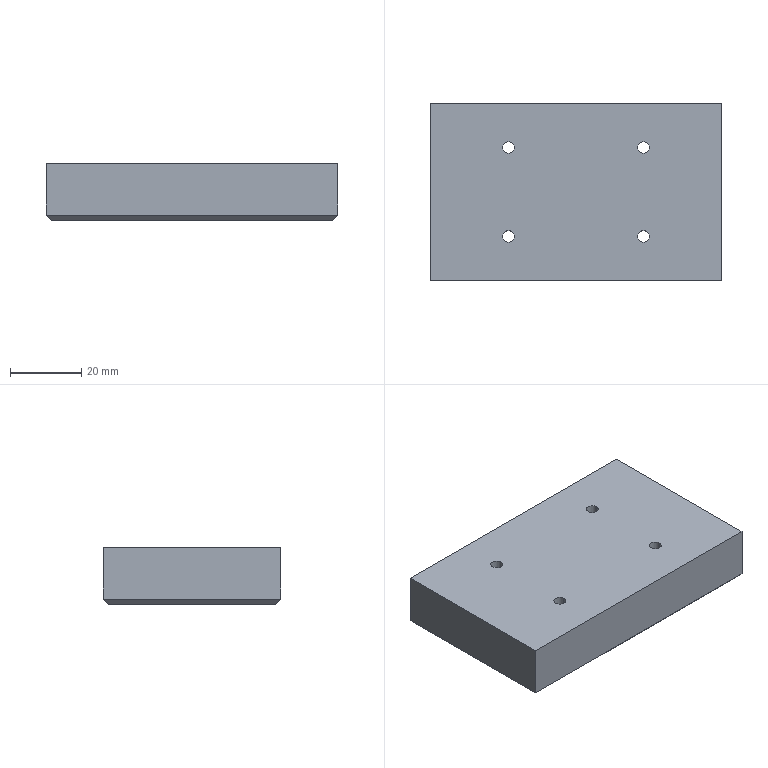Part | SolidWorks | features 3DProfileFeature 1, Chamfer 1, Extrusion 1, HoleWzd 1, LPattern 1 | 1 solid | 18 faces | box 82 x 50 x 16 mm | volume 64760 mm3 | plane 10 | cylinder 8 | commonest cylinder face diameters 3.3 x8
STEP:
#1=CARTESIAN_POINT('',(-17.35,-12.5,16.));
#2=VERTEX_POINT('',#1);
#3=CARTESIAN_POINT('',(-20.65,-12.5,16.));
#4=VERTEX_POINT('',#3);
#5=CARTESIAN_POINT('',(-19.,-12.5,16.));
#6=DIRECTION('',(0.,0.,-1.));
#7=DIRECTION('',(-1.,0.,0.));
#8=AXIS2_PLACEMENT_3D('',#5,#6,#7);
#9=CIRCLE('',#8,1.65);
#10=EDGE_CURVE('',#2,#4,#9,.T.);
#11=ORIENTED_EDGE('',*,*,#10,.F.);
#12=CARTESIAN_POINT('',(-17.35,-12.5,0.));
#13=VERTEX_POINT('',#12);
#14=CARTESIAN_POINT('',(-17.35,-12.5,0.));
#15=DIRECTION('',(0.,0.,-1.));
#16=VECTOR('',#15,1000.);
#17=LINE('',#14,#16);
#18=EDGE_CURVE('',#2,#13,#17,.T.);
#19=ORIENTED_EDGE('',*,*,#18,.T.);
#20=CARTESIAN_POINT('',(-20.65,-12.5,0.));
#21=VERTEX_POINT('',#20);
#22=CARTESIAN_POINT('',(-19.,-12.5,0.));
#23=DIRECTION('',(0.,0.,-1.));
#24=DIRECTION('',(-1.,0.,0.));
#25=AXIS2_PLACEMENT_3D('',#22,#23,#24);
#26=CIRCLE('',#25,1.65);
#27=EDGE_CURVE('',#13,#21,#26,.T.);
#28=ORIENTED_EDGE('',*,*,#27,.T.);
#29=CARTESIAN_POINT('',(-20.65,-12.5,0.));
#30=DIRECTION('',(0.,0.,-1.));
#31=VECTOR('',#30,1000.);
#32=LINE('',#29,#31);
#33=EDGE_CURVE('',#4,#21,#32,.T.);
#34=ORIENTED_EDGE('',*,*,#33,.F.);
#35=EDGE_LOOP('',(#11,#19,#28,#34));
#36=FACE_OUTER_BOUND('',#35,.T.);
#37=CARTESIAN_POINT('',(-19.,-12.5,0.));
#38=DIRECTION('',(0.,0.,-1.));
#39=DIRECTION('',(-1.,0.,0.));
#40=AXIS2_PLACEMENT_3D('',#37,#38,#39);
#41=CYLINDRICAL_SURFACE('',#40,1.65);
#42=ADVANCED_FACE('',(#36),#41,.F.);
#43=CARTESIAN_POINT('',(-17.35,12.5,16.));
#44=VERTEX_POINT('',#43);
#45=CARTESIAN_POINT('',(-20.65,12.5,16.));
#46=VERTEX_POINT('',#45);
#47=CARTESIAN_POINT('',(-19.,12.5,16.));
#48=DIRECTION('',(0.,0.,-1.));
#49=DIRECTION('',(-1.,0.,0.));
#50=AXIS2_PLACEMENT_3D('',#47,#48,#49);
#51=CIRCLE('',#50,1.65);
#52=EDGE_CURVE('',#44,#46,#51,.T.);
#53=ORIENTED_EDGE('',*,*,#52,.F.);
#54=CARTESIAN_POINT('',(-17.35,12.5,0.));
#55=VERTEX_POINT('',#54);
#56=CARTESIAN_POINT('',(-17.35,12.5,0.));
#57=DIRECTION('',(0.,0.,-1.));
#58=VECTOR('',#57,1000.);
#59=LINE('',#56,#58);
#60=EDGE_CURVE('',#44,#55,#59,.T.);
#61=ORIENTED_EDGE('',*,*,#60,.T.);
#62=CARTESIAN_POINT('',(-20.65,12.5,0.));
#63=VERTEX_POINT('',#62);
#64=CARTESIAN_POINT('',(-19.,12.5,0.));
#65=DIRECTION('',(0.,0.,-1.));
#66=DIRECTION('',(-1.,0.,0.));
#67=AXIS2_PLACEMENT_3D('',#64,#65,#66);
#68=CIRCLE('',#67,1.65);
#69=EDGE_CURVE('',#55,#63,#68,.T.);
#70=ORIENTED_EDGE('',*,*,#69,.T.);
#71=CARTESIAN_POINT('',(-20.65,12.5,0.));
#72=DIRECTION('',(0.,0.,-1.));
#73=VECTOR('',#72,1000.);
#74=LINE('',#71,#73);
#75=EDGE_CURVE('',#46,#63,#74,.T.);
#76=ORIENTED_EDGE('',*,*,#75,.F.);
#77=EDGE_LOOP('',(#53,#61,#70,#76));
#78=FACE_OUTER_BOUND('',#77,.T.);
#79=CARTESIAN_POINT('',(-19.,12.5,0.));
#80=DIRECTION('',(0.,0.,-1.));
#81=DIRECTION('',(-1.,0.,0.));
#82=AXIS2_PLACEMENT_3D('',#79,#80,#81);
#83=CYLINDRICAL_SURFACE('',#82,1.65);
#84=ADVANCED_FACE('',(#78),#83,.F.);
#85=CARTESIAN_POINT('',(20.65,-12.5,16.));
#86=VERTEX_POINT('',#85);
#87=CARTESIAN_POINT('',(17.35,-12.5,16.));
#88=VERTEX_POINT('',#87);
#89=CARTESIAN_POINT('',(19.,-12.5,16.));
#90=DIRECTION('',(0.,0.,-1.));
#91=DIRECTION('',(-1.,0.,0.));
#92=AXIS2_PLACEMENT_3D('',#89,#90,#91);
#93=CIRCLE('',#92,1.65);
#94=EDGE_CURVE('',#86,#88,#93,.T.);
#95=ORIENTED_EDGE('',*,*,#94,.F.);
#96=CARTESIAN_POINT('',(20.65,-12.5,0.));
#97=VERTEX_POINT('',#96);
#98=CARTESIAN_POINT('',(20.65,-12.5,0.));
#99=DIRECTION('',(0.,0.,-1.));
#100=VECTOR('',#99,1000.);
#101=LINE('',#98,#100);
#102=EDGE_CURVE('',#86,#97,#101,.T.);
#103=ORIENTED_EDGE('',*,*,#102,.T.);
#104=CARTESIAN_POINT('',(17.35,-12.5,0.));
#105=VERTEX_POINT('',#104);
#106=CARTESIAN_POINT('',(19.,-12.5,0.));
#107=DIRECTION('',(0.,0.,-1.));
#108=DIRECTION('',(-1.,0.,0.));
#109=AXIS2_PLACEMENT_3D('',#106,#107,#108);
#110=CIRCLE('',#109,1.65);
#111=EDGE_CURVE('',#97,#105,#110,.T.);
#112=ORIENTED_EDGE('',*,*,#111,.T.);
#113=CARTESIAN_POINT('',(17.35,-12.5,0.));
#114=DIRECTION('',(0.,0.,-1.));
#115=VECTOR('',#114,1000.);
#116=LINE('',#113,#115);
#117=EDGE_CURVE('',#88,#105,#116,.T.);
#118=ORIENTED_EDGE('',*,*,#117,.F.);
#119=EDGE_LOOP('',(#95,#103,#112,#118));
#120=FACE_OUTER_BOUND('',#119,.T.);
#121=CARTESIAN_POINT('',(19.,-12.5,0.));
#122=DIRECTION('',(0.,0.,-1.));
#123=DIRECTION('',(-1.,0.,0.));
#124=AXIS2_PLACEMENT_3D('',#121,#122,#123);
#125=CYLINDRICAL_SURFACE('',#124,1.65);
#126=ADVANCED_FACE('',(#120),#125,.F.);
#127=CARTESIAN_POINT('',(20.65,12.5,16.));
#128=VERTEX_POINT('',#127);
#129=CARTESIAN_POINT('',(17.35,12.5,16.));
#130=VERTEX_POINT('',#129);
#131=CARTESIAN_POINT('',(19.,12.5,16.));
#132=DIRECTION('',(0.,0.,-1.));
#133=DIRECTION('',(-1.,0.,0.));
#134=AXIS2_PLACEMENT_3D('',#131,#132,#133);
#135=CIRCLE('',#134,1.65);
#136=EDGE_CURVE('',#128,#130,#135,.T.);
#137=ORIENTED_EDGE('',*,*,#136,.F.);
#138=CARTESIAN_POINT('',(20.65,12.5,0.));
#139=VERTEX_POINT('',#138);
#140=CARTESIAN_POINT('',(20.65,12.5,0.));
#141=DIRECTION('',(0.,0.,-1.));
#142=VECTOR('',#141,1000.);
#143=LINE('',#140,#142);
#144=EDGE_CURVE('',#128,#139,#143,.T.);
#145=ORIENTED_EDGE('',*,*,#144,.T.);
#146=CARTESIAN_POINT('',(17.35,12.5,0.));
#147=VERTEX_POINT('',#146);
#148=CARTESIAN_POINT('',(19.,12.5,0.));
#149=DIRECTION('',(0.,0.,-1.));
#150=DIRECTION('',(-1.,0.,0.));
#151=AXIS2_PLACEMENT_3D('',#148,#149,#150);
#152=CIRCLE('',#151,1.65);
#153=EDGE_CURVE('',#139,#147,#152,.T.);
#154=ORIENTED_EDGE('',*,*,#153,.T.);
#155=CARTESIAN_POINT('',(17.35,12.5,0.));
#156=DIRECTION('',(0.,0.,-1.));
#157=VECTOR('',#156,1000.);
#158=LINE('',#155,#157);
#159=EDGE_CURVE('',#130,#147,#158,.T.);
#160=ORIENTED_EDGE('',*,*,#159,.F.);
#161=EDGE_LOOP('',(#137,#145,#154,#160));
#162=FACE_OUTER_BOUND('',#161,.T.);
#163=CARTESIAN_POINT('',(19.,12.5,0.));
#164=DIRECTION('',(0.,0.,-1.));
#165=DIRECTION('',(-1.,0.,0.));
#166=AXIS2_PLACEMENT_3D('',#163,#164,#165);
#167=CYLINDRICAL_SURFACE('',#166,1.65);
#168=ADVANCED_FACE('',(#162),#167,.F.);
#169=CARTESIAN_POINT('',(-41.,25.,16.));
#170=VERTEX_POINT('',#169);
#171=CARTESIAN_POINT('',(-41.,25.,1.5));
#172=VERTEX_POINT('',#171);
#173=CARTESIAN_POINT('',(-41.,25.,16.));
#174=DIRECTION('',(0.,0.,-1.));
#175=VECTOR('',#174,1000.);
#176=LINE('',#173,#175);
#177=EDGE_CURVE('',#170,#172,#176,.T.);
#178=ORIENTED_EDGE('',*,*,#177,.T.);
#179=CARTESIAN_POINT('',(-41.,-25.,1.5));
#180=VERTEX_POINT('',#179);
#181=CARTESIAN_POINT('',(-41.,-25.,1.5));
#182=DIRECTION('',(0.,-1.,0.));
#183=VECTOR('',#182,1000.);
#184=LINE('',#181,#183);
#185=EDGE_CURVE('',#172,#180,#184,.T.);
#186=ORIENTED_EDGE('',*,*,#185,.T.);
#187=CARTESIAN_POINT('',(-41.,-25.,16.));
#188=VERTEX_POINT('',#187);
#189=CARTESIAN_POINT('',(-41.,-25.,16.));
#190=DIRECTION('',(0.,0.,-1.));
#191=VECTOR('',#190,1000.);
#192=LINE('',#189,#191);
#193=EDGE_CURVE('',#188,#180,#192,.T.);
#194=ORIENTED_EDGE('',*,*,#193,.F.);
#195=CARTESIAN_POINT('',(-41.,25.,16.));
#196=DIRECTION('',(0.,-1.,0.));
#197=VECTOR('',#196,1000.);
#198=LINE('',#195,#197);
#199=EDGE_CURVE('',#170,#188,#198,.T.);
#200=ORIENTED_EDGE('',*,*,#199,.F.);
#201=EDGE_LOOP('',(#178,#186,#194,#200));
#202=FACE_OUTER_BOUND('',#201,.T.);
#203=CARTESIAN_POINT('',(-41.,25.,16.));
#204=DIRECTION('',(1.,0.,0.));
#205=DIRECTION('',(0.,0.,-1.));
#206=AXIS2_PLACEMENT_3D('',#203,#204,#205);
#207=PLANE('',#206);
#208=ADVANCED_FACE('',(#202),#207,.F.);
#209=ORIENTED_EDGE('',*,*,#193,.T.);
#210=CARTESIAN_POINT('',(41.,-25.,1.5));
#211=VERTEX_POINT('',#210);
#212=CARTESIAN_POINT('',(41.,-25.,1.5));
#213=DIRECTION('',(1.,0.,0.));
#214=VECTOR('',#213,1000.);
#215=LINE('',#212,#214);
#216=EDGE_CURVE('',#180,#211,#215,.T.);
#217=ORIENTED_EDGE('',*,*,#216,.T.);
#218=CARTESIAN_POINT('',(41.,-25.,16.));
#219=VERTEX_POINT('',#218);
#220=CARTESIAN_POINT('',(41.,-25.,16.));
#221=DIRECTION('',(0.,0.,-1.));
#222=VECTOR('',#221,1000.);
#223=LINE('',#220,#222);
#224=EDGE_CURVE('',#219,#211,#223,.T.);
#225=ORIENTED_EDGE('',*,*,#224,.F.);
#226=CARTESIAN_POINT('',(41.,-25.,16.));
#227=DIRECTION('',(1.,0.,0.));
#228=VECTOR('',#227,1000.);
#229=LINE('',#226,#228);
#230=EDGE_CURVE('',#188,#219,#229,.T.);
#231=ORIENTED_EDGE('',*,*,#230,.F.);
#232=EDGE_LOOP('',(#209,#217,#225,#231));
#233=FACE_OUTER_BOUND('',#232,.T.);
#234=CARTESIAN_POINT('',(41.,-25.,16.));
#235=DIRECTION('',(0.,1.,0.));
#236=DIRECTION('',(-1.,0.,0.));
#237=AXIS2_PLACEMENT_3D('',#234,#235,#236);
#238=PLANE('',#237);
#239=ADVANCED_FACE('',(#233),#238,.F.);
#240=ORIENTED_EDGE('',*,*,#224,.T.);
#241=CARTESIAN_POINT('',(41.,25.,1.5));
#242=VERTEX_POINT('',#241);
#243=CARTESIAN_POINT('',(41.,25.,1.5));
#244=DIRECTION('',(0.,1.,0.));
#245=VECTOR('',#244,1000.);
#246=LINE('',#243,#245);
#247=EDGE_CURVE('',#211,#242,#246,.T.);
#248=ORIENTED_EDGE('',*,*,#247,.T.);
#249=CARTESIAN_POINT('',(41.,25.,16.));
#250=VERTEX_POINT('',#249);
#251=CARTESIAN_POINT('',(41.,25.,16.));
#252=DIRECTION('',(0.,0.,-1.));
#253=VECTOR('',#252,1000.);
#254=LINE('',#251,#253);
#255=EDGE_CURVE('',#250,#242,#254,.T.);
#256=ORIENTED_EDGE('',*,*,#255,.F.);
#257=CARTESIAN_POINT('',(41.,25.,16.));
#258=DIRECTION('',(0.,1.,0.));
#259=VECTOR('',#258,1000.);
#260=LINE('',#257,#259);
#261=EDGE_CURVE('',#219,#250,#260,.T.);
#262=ORIENTED_EDGE('',*,*,#261,.F.);
#263=EDGE_LOOP('',(#240,#248,#256,#262));
#264=FACE_OUTER_BOUND('',#263,.T.);
#265=CARTESIAN_POINT('',(41.,25.,16.));
#266=DIRECTION('',(-1.,0.,0.));
#267=DIRECTION('',(0.,0.,1.));
#268=AXIS2_PLACEMENT_3D('',#265,#266,#267);
#269=PLANE('',#268);
#270=ADVANCED_FACE('',(#264),#269,.F.);
#271=ORIENTED_EDGE('',*,*,#255,.T.);
#272=CARTESIAN_POINT('',(-41.,25.,1.5));
#273=DIRECTION('',(-1.,0.,0.));
#274=VECTOR('',#273,1000.);
#275=LINE('',#272,#274);
#276=EDGE_CURVE('',#242,#172,#275,.T.);
#277=ORIENTED_EDGE('',*,*,#276,.T.);
#278=ORIENTED_EDGE('',*,*,#177,.F.);
#279=CARTESIAN_POINT('',(41.,25.,16.));
#280=DIRECTION('',(-1.,0.,0.));
#281=VECTOR('',#280,1000.);
#282=LINE('',#279,#281);
#283=EDGE_CURVE('',#250,#170,#282,.T.);
#284=ORIENTED_EDGE('',*,*,#283,.F.);
#285=EDGE_LOOP('',(#271,#277,#278,#284));
#286=FACE_OUTER_BOUND('',#285,.T.);
#287=CARTESIAN_POINT('',(41.,25.,16.));
#288=DIRECTION('',(0.,-1.,0.));
#289=DIRECTION('',(1.,0.,0.));
#290=AXIS2_PLACEMENT_3D('',#287,#288,#289);
#291=PLANE('',#290);
#292=ADVANCED_FACE('',(#286),#291,.F.);
#293=CARTESIAN_POINT('',(-19.,-12.5,16.));
#294=DIRECTION('',(0.,0.,-1.));
#295=DIRECTION('',(-1.,0.,0.));
#296=AXIS2_PLACEMENT_3D('',#293,#294,#295);
#297=CIRCLE('',#296,1.65);
#298=EDGE_CURVE('',#4,#2,#297,.T.);
#299=ORIENTED_EDGE('',*,*,#298,.T.);
#300=ORIENTED_EDGE('',*,*,#10,.T.);
#301=EDGE_LOOP('',(#299,#300));
#302=FACE_BOUND('',#301,.T.);
#303=CARTESIAN_POINT('',(-19.,12.5,16.));
#304=DIRECTION('',(0.,0.,-1.));
#305=DIRECTION('',(-1.,0.,0.));
#306=AXIS2_PLACEMENT_3D('',#303,#304,#305);
#307=CIRCLE('',#306,1.65);
#308=EDGE_CURVE('',#46,#44,#307,.T.);
#309=ORIENTED_EDGE('',*,*,#308,.T.);
#310=ORIENTED_EDGE('',*,*,#52,.T.);
#311=EDGE_LOOP('',(#309,#310));
#312=FACE_BOUND('',#311,.T.);
#313=CARTESIAN_POINT('',(19.,-12.5,16.));
#314=DIRECTION('',(0.,0.,-1.));
#315=DIRECTION('',(-1.,0.,0.));
#316=AXIS2_PLACEMENT_3D('',#313,#314,#315);
#317=CIRCLE('',#316,1.65);
#318=EDGE_CURVE('',#88,#86,#317,.T.);
#319=ORIENTED_EDGE('',*,*,#318,.T.);
#320=ORIENTED_EDGE('',*,*,#94,.T.);
#321=EDGE_LOOP('',(#319,#320));
#322=FACE_BOUND('',#321,.T.);
#323=CARTESIAN_POINT('',(19.,12.5,16.));
#324=DIRECTION('',(0.,0.,-1.));
#325=DIRECTION('',(-1.,0.,0.));
#326=AXIS2_PLACEMENT_3D('',#323,#324,#325);
#327=CIRCLE('',#326,1.65);
#328=EDGE_CURVE('',#130,#128,#327,.T.);
#329=ORIENTED_EDGE('',*,*,#328,.T.);
#330=ORIENTED_EDGE('',*,*,#136,.T.);
#331=EDGE_LOOP('',(#329,#330));
#332=FACE_BOUND('',#331,.T.);
#333=ORIENTED_EDGE('',*,*,#199,.T.);
#334=ORIENTED_EDGE('',*,*,#230,.T.);
#335=ORIENTED_EDGE('',*,*,#261,.T.);
#336=ORIENTED_EDGE('',*,*,#283,.T.);
#337=EDGE_LOOP('',(#333,#334,#335,#336));
#338=FACE_OUTER_BOUND('',#337,.T.);
#339=CARTESIAN_POINT('',(0.,0.,16.));
#340=DIRECTION('',(0.,0.,-1.));
#341=DIRECTION('',(-1.,0.,0.));
#342=AXIS2_PLACEMENT_3D('',#339,#340,#341);
#343=PLANE('',#342);
#344=ADVANCED_FACE('',(#302,#312,#322,#332,#338),#343,.F.);
#345=CARTESIAN_POINT('',(39.5,-23.5,0.));
#346=VERTEX_POINT('',#345);
#347=CARTESIAN_POINT('',(-39.5,-23.5,0.));
#348=VERTEX_POINT('',#347);
#349=CARTESIAN_POINT('',(-41.,-23.5,0.));
#350=DIRECTION('',(-1.,0.,0.));
#351=VECTOR('',#350,1000.);
#352=LINE('',#349,#351);
#353=EDGE_CURVE('',#346,#348,#352,.T.);
#354=ORIENTED_EDGE('',*,*,#353,.T.);
#355=CARTESIAN_POINT('',(-39.5,23.5,0.));
#356=VERTEX_POINT('',#355);
#357=CARTESIAN_POINT('',(-39.5,25.,0.));
#358=DIRECTION('',(0.,1.,0.));
#359=VECTOR('',#358,1000.);
#360=LINE('',#357,#359);
#361=EDGE_CURVE('',#348,#356,#360,.T.);
#362=ORIENTED_EDGE('',*,*,#361,.T.);
#363=CARTESIAN_POINT('',(39.5,23.5,0.));
#364=VERTEX_POINT('',#363);
#365=CARTESIAN_POINT('',(41.,23.5,0.));
#366=DIRECTION('',(1.,0.,0.));
#367=VECTOR('',#366,1000.);
#368=LINE('',#365,#367);
#369=EDGE_CURVE('',#356,#364,#368,.T.);
#370=ORIENTED_EDGE('',*,*,#369,.T.);
#371=CARTESIAN_POINT('',(39.5,-25.,0.));
#372=DIRECTION('',(0.,-1.,0.));
#373=VECTOR('',#372,1000.);
#374=LINE('',#371,#373);
#375=EDGE_CURVE('',#364,#346,#374,.T.);
#376=ORIENTED_EDGE('',*,*,#375,.T.);
#377=EDGE_LOOP('',(#354,#362,#370,#376));
#378=FACE_OUTER_BOUND('',#377,.T.);
#379=CARTESIAN_POINT('',(-19.,-12.5,0.));
#380=DIRECTION('',(0.,0.,-1.));
#381=DIRECTION('',(-1.,0.,0.));
#382=AXIS2_PLACEMENT_3D('',#379,#380,#381);
#383=CIRCLE('',#382,1.65);
#384=EDGE_CURVE('',#21,#13,#383,.T.);
#385=ORIENTED_EDGE('',*,*,#384,.F.);
#386=ORIENTED_EDGE('',*,*,#27,.F.);
#387=EDGE_LOOP('',(#385,#386));
#388=FACE_BOUND('',#387,.T.);
#389=CARTESIAN_POINT('',(-19.,12.5,0.));
#390=DIRECTION('',(0.,0.,-1.));
#391=DIRECTION('',(-1.,0.,0.));
#392=AXIS2_PLACEMENT_3D('',#389,#390,#391);
#393=CIRCLE('',#392,1.65);
#394=EDGE_CURVE('',#63,#55,#393,.T.);
#395=ORIENTED_EDGE('',*,*,#394,.F.);
#396=ORIENTED_EDGE('',*,*,#69,.F.);
#397=EDGE_LOOP('',(#395,#396));
#398=FACE_BOUND('',#397,.T.);
#399=CARTESIAN_POINT('',(19.,-12.5,0.));
#400=DIRECTION('',(0.,0.,-1.));
#401=DIRECTION('',(-1.,0.,0.));
#402=AXIS2_PLACEMENT_3D('',#399,#400,#401);
#403=CIRCLE('',#402,1.65);
#404=EDGE_CURVE('',#105,#97,#403,.T.);
#405=ORIENTED_EDGE('',*,*,#404,.F.);
#406=ORIENTED_EDGE('',*,*,#111,.F.);
#407=EDGE_LOOP('',(#405,#406));
#408=FACE_BOUND('',#407,.T.);
#409=CARTESIAN_POINT('',(19.,12.5,0.));
#410=DIRECTION('',(0.,0.,-1.));
#411=DIRECTION('',(-1.,0.,0.));
#412=AXIS2_PLACEMENT_3D('',#409,#410,#411);
#413=CIRCLE('',#412,1.65);
#414=EDGE_CURVE('',#147,#139,#413,.T.);
#415=ORIENTED_EDGE('',*,*,#414,.F.);
#416=ORIENTED_EDGE('',*,*,#153,.F.);
#417=EDGE_LOOP('',(#415,#416));
#418=FACE_BOUND('',#417,.T.);
#419=CARTESIAN_POINT('',(0.,0.,0.));
#420=DIRECTION('',(0.,0.,-1.));
#421=DIRECTION('',(-1.,0.,0.));
#422=AXIS2_PLACEMENT_3D('',#419,#420,#421);
#423=PLANE('',#422);
#424=ADVANCED_FACE('',(#378,#388,#398,#408,#418),#423,.T.);
#425=ORIENTED_EDGE('',*,*,#144,.F.);
#426=ORIENTED_EDGE('',*,*,#328,.F.);
#427=ORIENTED_EDGE('',*,*,#159,.T.);
#428=ORIENTED_EDGE('',*,*,#414,.T.);
#429=EDGE_LOOP('',(#425,#426,#427,#428));
#430=FACE_OUTER_BOUND('',#429,.T.);
#431=CARTESIAN_POINT('',(19.,12.5,0.));
#432=DIRECTION('',(0.,0.,-1.));
#433=DIRECTION('',(-1.,0.,0.));
#434=AXIS2_PLACEMENT_3D('',#431,#432,#433);
#435=CYLINDRICAL_SURFACE('',#434,1.65);
#436=ADVANCED_FACE('',(#430),#435,.F.);
#437=ORIENTED_EDGE('',*,*,#102,.F.);
#438=ORIENTED_EDGE('',*,*,#318,.F.);
#439=ORIENTED_EDGE('',*,*,#117,.T.);
#440=ORIENTED_EDGE('',*,*,#404,.T.);
#441=EDGE_LOOP('',(#437,#438,#439,#440));
#442=FACE_OUTER_BOUND('',#441,.T.);
#443=CARTESIAN_POINT('',(19.,-12.5,0.));
#444=DIRECTION('',(0.,0.,-1.));
#445=DIRECTION('',(-1.,0.,0.));
#446=AXIS2_PLACEMENT_3D('',#443,#444,#445);
#447=CYLINDRICAL_SURFACE('',#446,1.65);
#448=ADVANCED_FACE('',(#442),#447,.F.);
#449=ORIENTED_EDGE('',*,*,#60,.F.);
#450=ORIENTED_EDGE('',*,*,#308,.F.);
#451=ORIENTED_EDGE('',*,*,#75,.T.);
#452=ORIENTED_EDGE('',*,*,#394,.T.);
#453=EDGE_LOOP('',(#449,#450,#451,#452));
#454=FACE_OUTER_BOUND('',#453,.T.);
#455=CARTESIAN_POINT('',(-19.,12.5,0.));
#456=DIRECTION('',(0.,0.,-1.));
#457=DIRECTION('',(-1.,0.,0.));
#458=AXIS2_PLACEMENT_3D('',#455,#456,#457);
#459=CYLINDRICAL_SURFACE('',#458,1.65);
#460=ADVANCED_FACE('',(#454),#459,.F.);
#461=ORIENTED_EDGE('',*,*,#18,.F.);
#462=ORIENTED_EDGE('',*,*,#298,.F.);
#463=ORIENTED_EDGE('',*,*,#33,.T.);
#464=ORIENTED_EDGE('',*,*,#384,.T.);
#465=EDGE_LOOP('',(#461,#462,#463,#464));
#466=FACE_OUTER_BOUND('',#465,.T.);
#467=CARTESIAN_POINT('',(-19.,-12.5,0.));
#468=DIRECTION('',(0.,0.,-1.));
#469=DIRECTION('',(-1.,0.,0.));
#470=AXIS2_PLACEMENT_3D('',#467,#468,#469);
#471=CYLINDRICAL_SURFACE('',#470,1.65);
#472=ADVANCED_FACE('',(#466),#471,.F.);
#473=CARTESIAN_POINT('',(24.333,-8.333,-15.167));
#474=DIRECTION('',(0.5774,-0.5774,0.5774));
#475=VECTOR('',#474,1000.);
#476=LINE('',#473,#475);
#477=EDGE_CURVE('',#346,#211,#476,.T.);
#478=ORIENTED_EDGE('',*,*,#477,.F.);
#479=ORIENTED_EDGE('',*,*,#375,.F.);
#480=CARTESIAN_POINT('',(41.,25.,1.5));
#481=DIRECTION('',(-0.5774,-0.5774,-0.5774));
#482=VECTOR('',#481,1000.);
#483=LINE('',#480,#482);
#484=EDGE_CURVE('',#242,#364,#483,.T.);
#485=ORIENTED_EDGE('',*,*,#484,.F.);
#486=ORIENTED_EDGE('',*,*,#247,.F.);
#487=EDGE_LOOP('',(#478,#479,#485,#486));
#488=FACE_OUTER_BOUND('',#487,.T.);
#489=CARTESIAN_POINT('',(41.,25.,1.5));
#490=DIRECTION('',(0.7071,0.,-0.7071));
#491=DIRECTION('',(0.,-1.,0.));
#492=AXIS2_PLACEMENT_3D('',#489,#490,#491);
#493=PLANE('',#492);
#494=ADVANCED_FACE('',(#488),#493,.T.);
#495=ORIENTED_EDGE('',*,*,#484,.T.);
#496=ORIENTED_EDGE('',*,*,#369,.F.);
#497=CARTESIAN_POINT('',(-13.667,-2.333,-25.833));
#498=DIRECTION('',(0.5774,-0.5774,-0.5774));
#499=VECTOR('',#498,1000.);
#500=LINE('',#497,#499);
#501=EDGE_CURVE('',#172,#356,#500,.T.);
#502=ORIENTED_EDGE('',*,*,#501,.F.);
#503=ORIENTED_EDGE('',*,*,#276,.F.);
#504=EDGE_LOOP('',(#495,#496,#502,#503));
#505=FACE_OUTER_BOUND('',#504,.T.);
#506=CARTESIAN_POINT('',(41.,25.,1.5));
#507=DIRECTION('',(0.,0.7071,-0.7071));
#508=DIRECTION('',(1.,0.,0.));
#509=AXIS2_PLACEMENT_3D('',#506,#507,#508);
#510=PLANE('',#509);
#511=ADVANCED_FACE('',(#505),#510,.T.);
#512=ORIENTED_EDGE('',*,*,#477,.T.);
#513=ORIENTED_EDGE('',*,*,#216,.F.);
#514=CARTESIAN_POINT('',(-13.667,2.333,-25.833));
#515=DIRECTION('',(-0.5774,-0.5774,0.5774));
#516=VECTOR('',#515,1000.);
#517=LINE('',#514,#516);
#518=EDGE_CURVE('',#348,#180,#517,.T.);
#519=ORIENTED_EDGE('',*,*,#518,.F.);
#520=ORIENTED_EDGE('',*,*,#353,.F.);
#521=EDGE_LOOP('',(#512,#513,#519,#520));
#522=FACE_OUTER_BOUND('',#521,.T.);
#523=CARTESIAN_POINT('',(41.,-25.,1.5));
#524=DIRECTION('',(0.,-0.7071,-0.7071));
#525=DIRECTION('',(-1.,0.,0.));
#526=AXIS2_PLACEMENT_3D('',#523,#524,#525);
#527=PLANE('',#526);
#528=ADVANCED_FACE('',(#522),#527,.T.);
#529=ORIENTED_EDGE('',*,*,#501,.T.);
#530=ORIENTED_EDGE('',*,*,#361,.F.);
#531=ORIENTED_EDGE('',*,*,#518,.T.);
#532=ORIENTED_EDGE('',*,*,#185,.F.);
#533=EDGE_LOOP('',(#529,#530,#531,#532));
#534=FACE_OUTER_BOUND('',#533,.T.);
#535=CARTESIAN_POINT('',(-41.,25.,1.5));
#536=DIRECTION('',(-0.7071,0.,-0.7071));
#537=DIRECTION('',(0.,1.,0.));
#538=AXIS2_PLACEMENT_3D('',#535,#536,#537);
#539=PLANE('',#538);
#540=ADVANCED_FACE('',(#534),#539,.T.);
#541=CLOSED_SHELL('',(#42,#84,#126,#168,#208,#239,#270,#292,#344,#424,#436,#448,#460,#472,#494,#511,#528,#540));
#542=MANIFOLD_SOLID_BREP('',#541);
#543=CARTESIAN_POINT('',(0.,0.,0.));
#544=DIRECTION('',(0.,0.,1.));
#545=DIRECTION('',(1.,0.,0.));
#546=AXIS2_PLACEMENT_3D('',#543,#544,#545);
#547=(LENGTH_UNIT()NAMED_UNIT(*)SI_UNIT(.MILLI.,.METRE.));
#548=UNCERTAINTY_MEASURE_WITH_UNIT(LENGTH_MEASURE(0.00001),#547,'','');
#549=(NAMED_UNIT(*)PLANE_ANGLE_UNIT()SI_UNIT($,.RADIAN.));
#550=(NAMED_UNIT(*)SI_UNIT($,.STERADIAN.)SOLID_ANGLE_UNIT());
#551=(GEOMETRIC_REPRESENTATION_CONTEXT(3)GLOBAL_UNCERTAINTY_ASSIGNED_CONTEXT((#548))GLOBAL_UNIT_ASSIGNED_CONTEXT((#547,#549,#550))REPRESENTATION_CONTEXT('',''));
#552=ADVANCED_BREP_SHAPE_REPRESENTATION('',(#542,#546),#551);